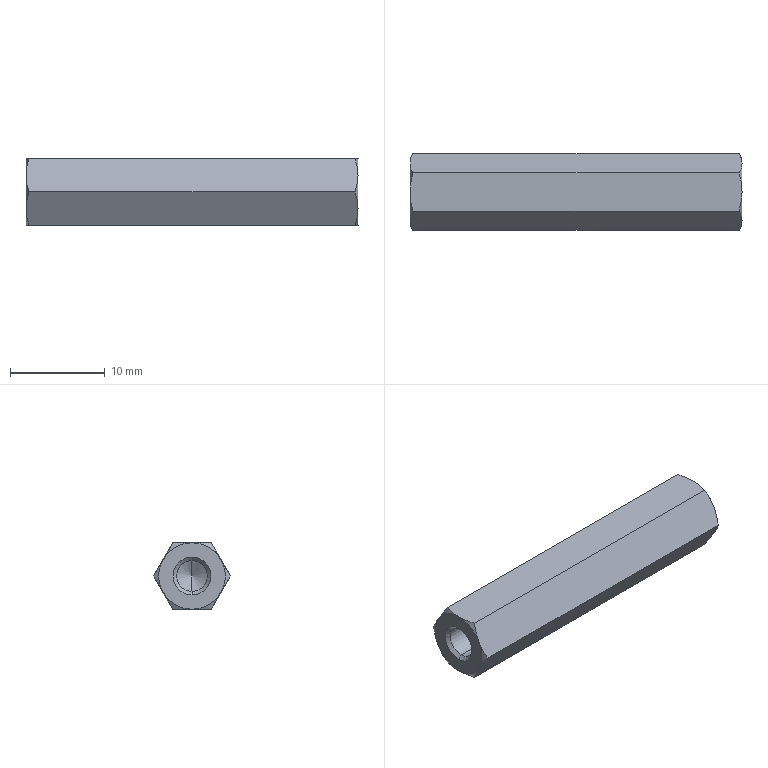Part | STEP file | 0243_005_PLSBRK7-35 | 1 solid | 32 faces | box 35 x 8.083 x 7 mm | volume 1328 mm3 | cone 20 | plane 8 | cylinder 4 | commonest cylinder face diameters 3.242 x4